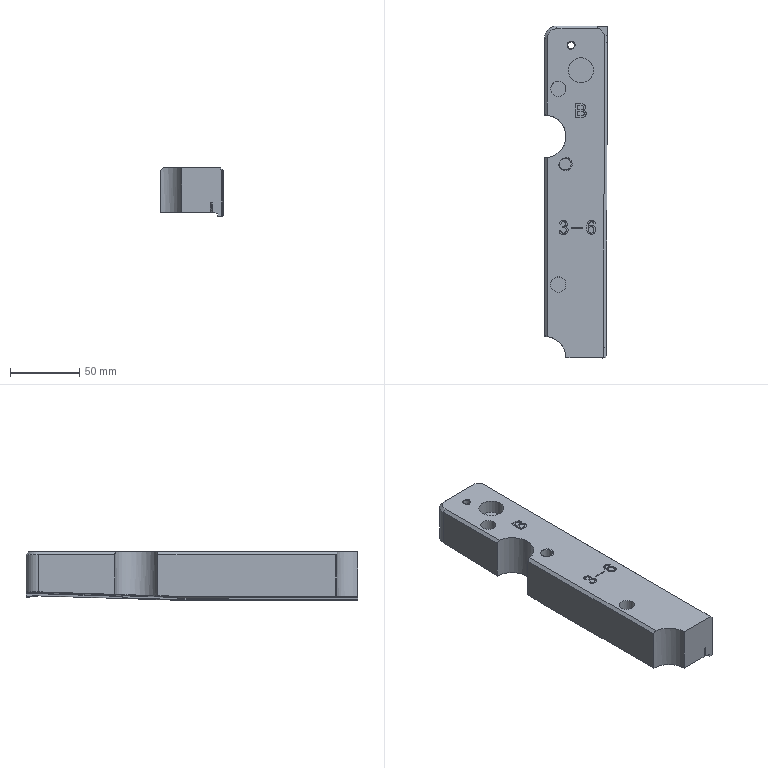Part | 1 solid | 176 faces | box 45.476 x 239.737 x 35.001 mm | volume 280724 mm3 | plane 96 | cylinder 54 | spline 22 | sphere 2 | cone 2 | commonest cylinder face diameters 1.006 x36 18 x5 10 x3 11 x2 31 x2 5 x1